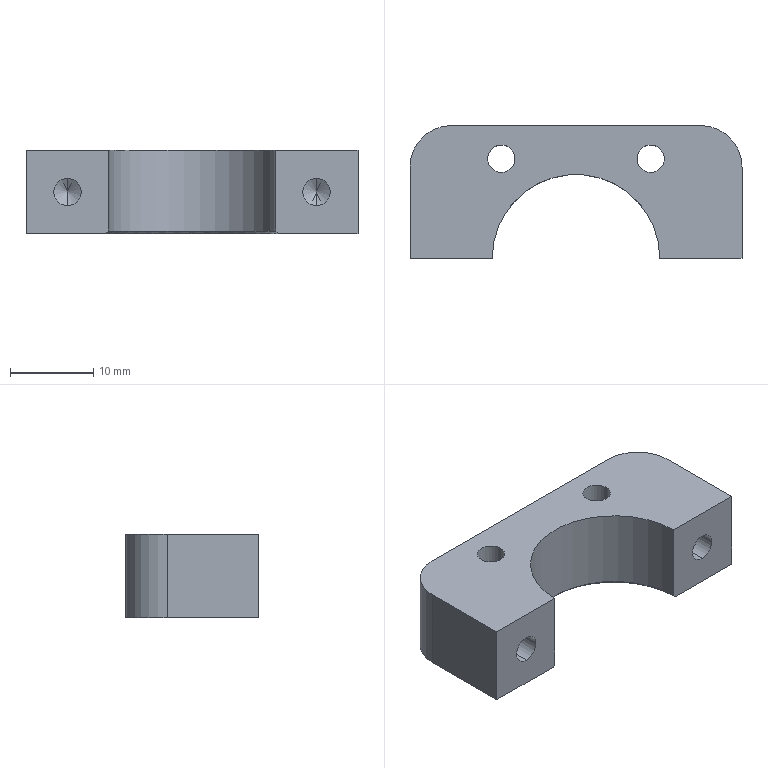Part | STEP file | photoelectric switch fixing plate 2 | 1 solid | 23 faces | box 40 x 16 x 10 mm | volume 4339 mm3 | cylinder 11 | plane 7 | cone 5 | commonest cylinder face diameters 3.3 x8 10 x2 20.2 x1